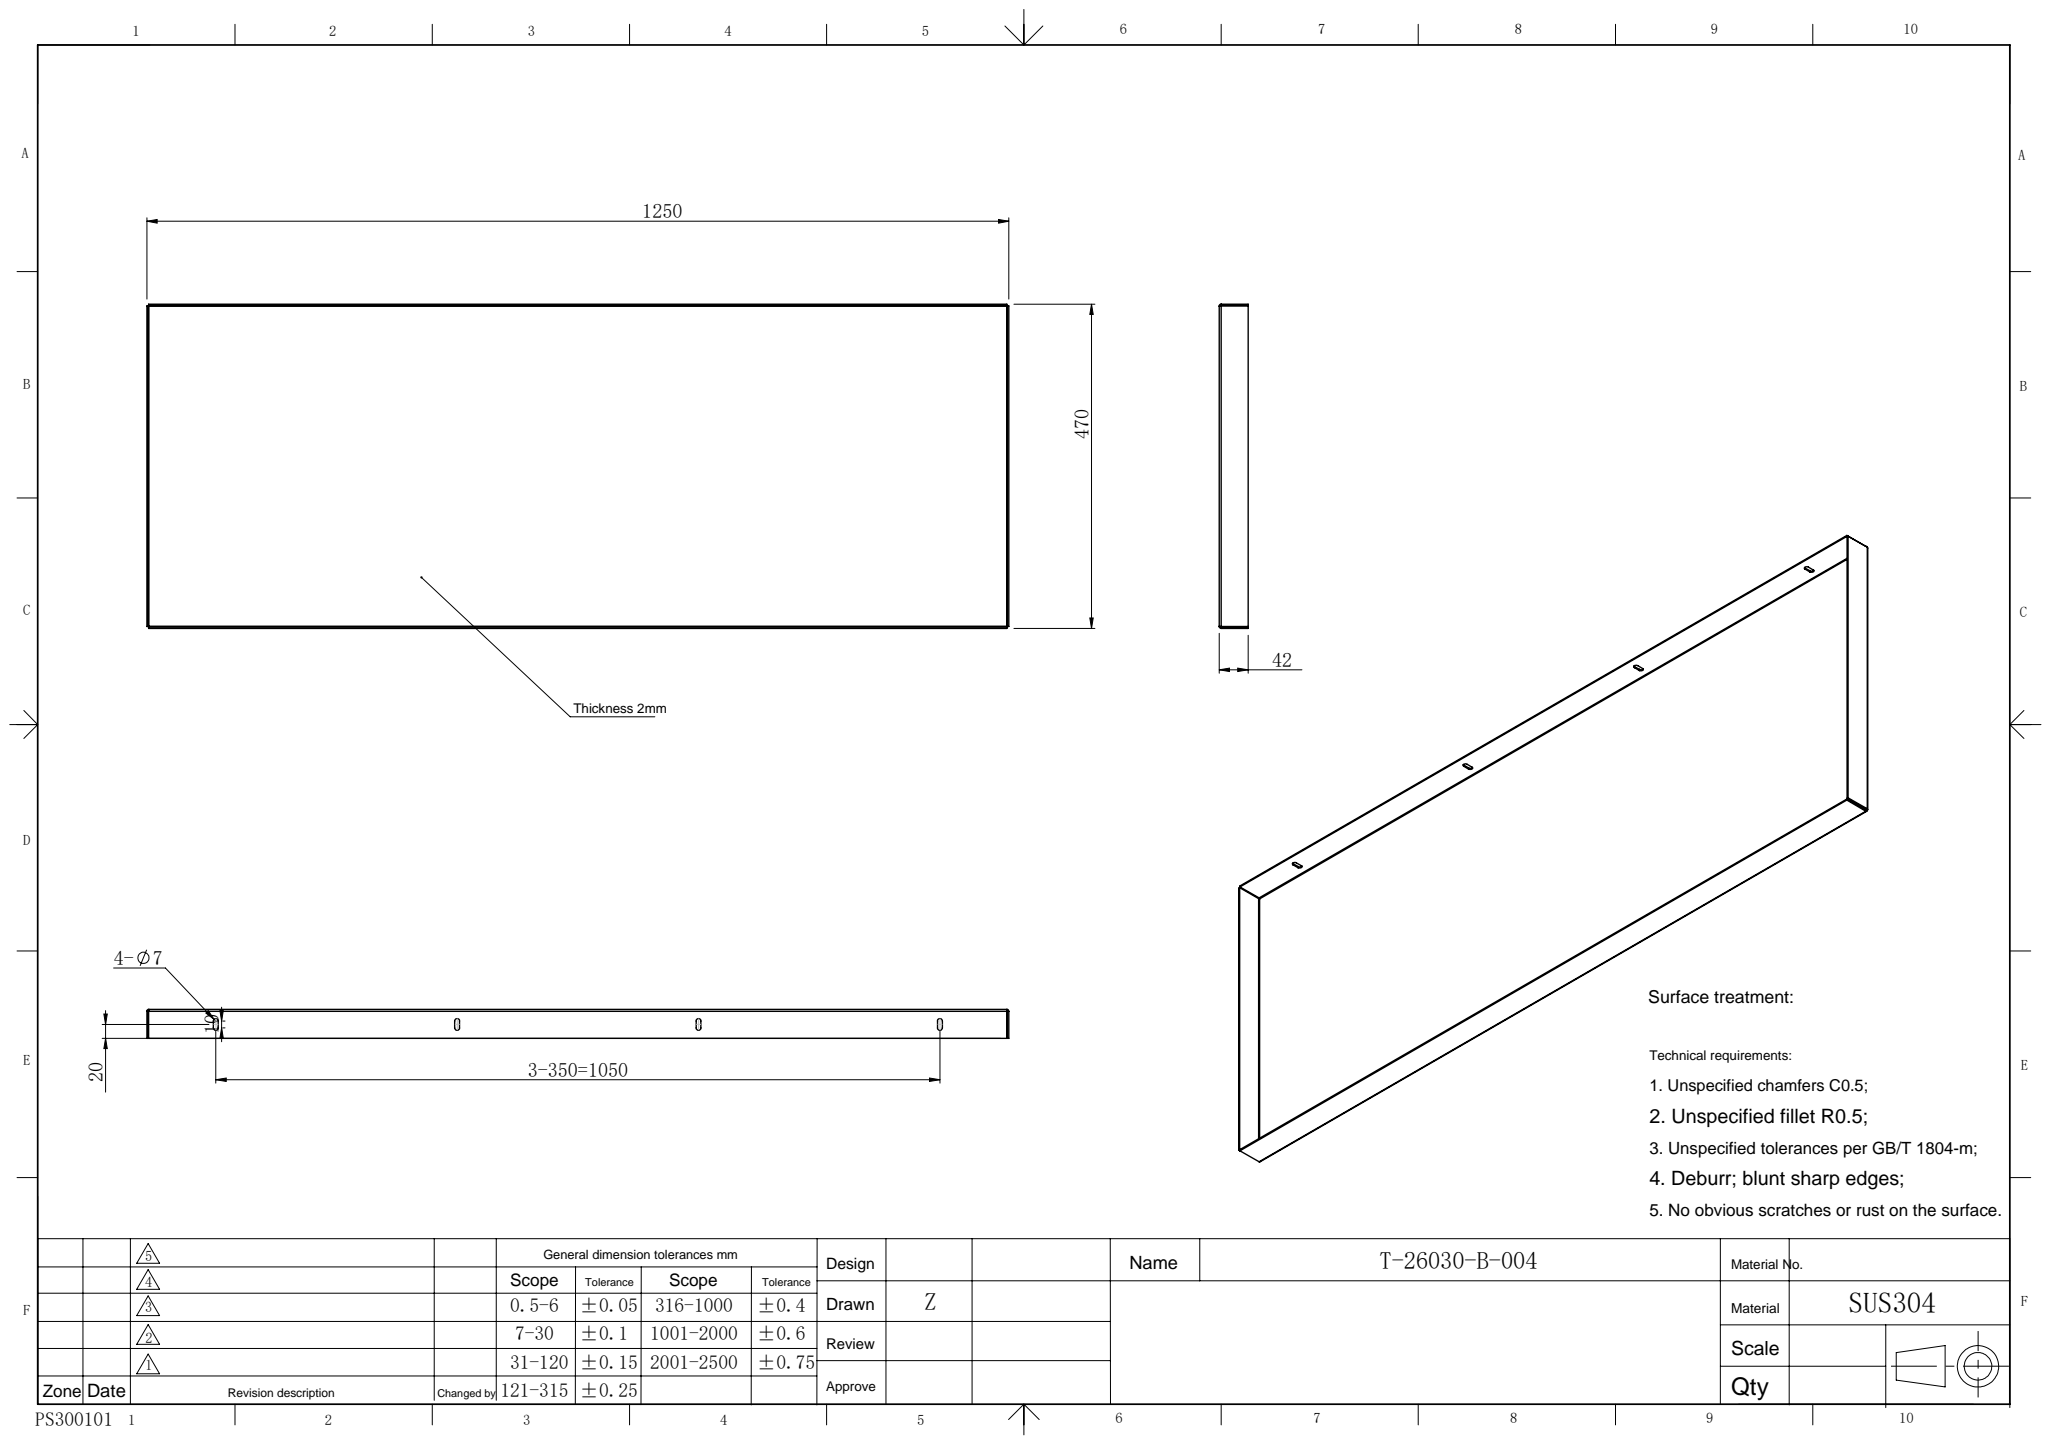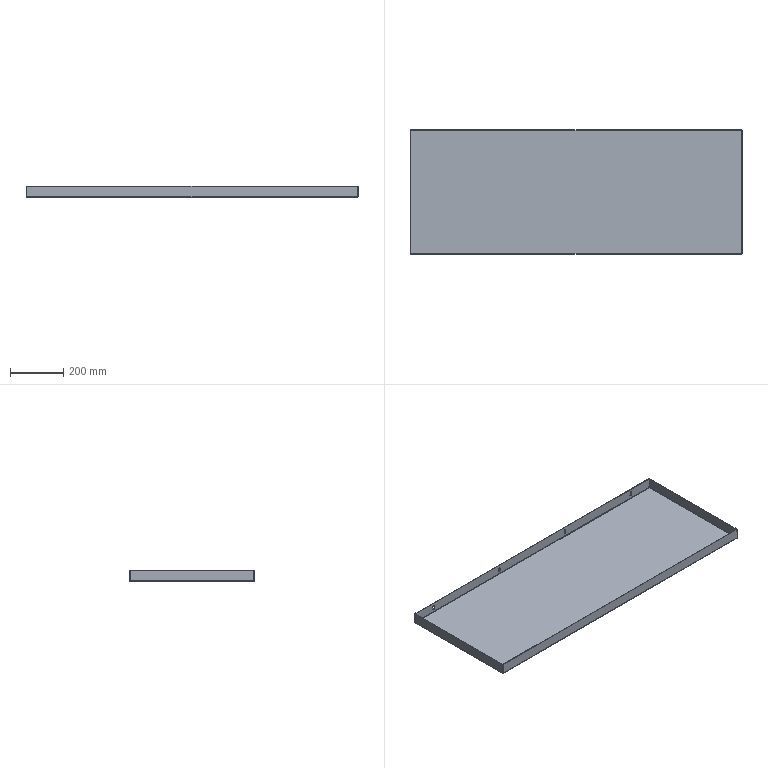Part | SolidWorks | features EdgeFlange 1, FlatPattern 1, ICE 1, LPattern 1, SMBaseFlange 1, SheetMetal 1 | 1 solid | 58 faces | box 1250 x 470 x 42 mm | volume 1441666 mm3 | plane 30 | cylinder 20 | spline 8 | commonest cylinder face diameters 7 x12 2 x4 6 x4